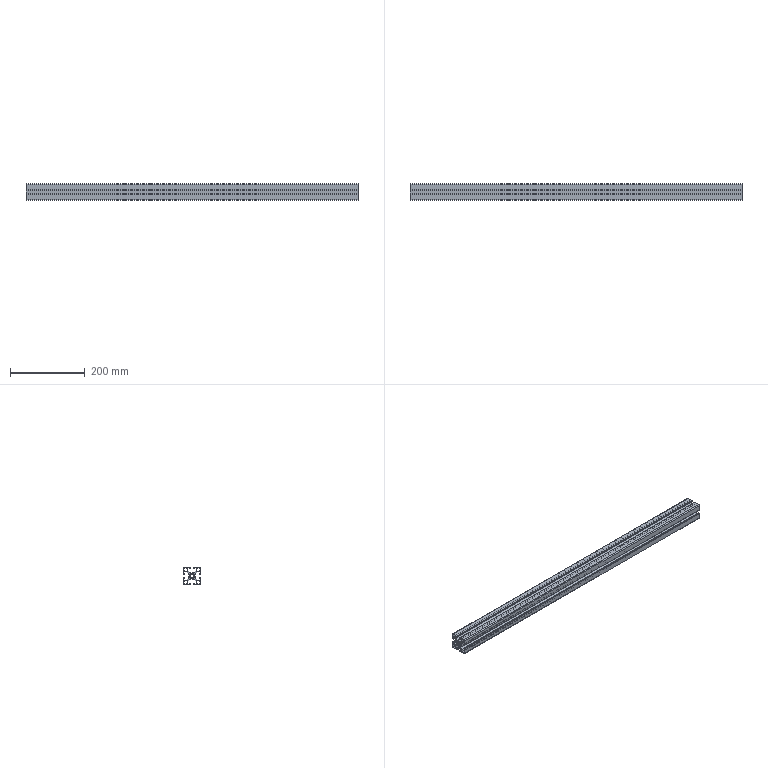Part | SolidWorks | features WeldMemberFeat 1, WeldmentFeature 1 | 1 solid | 135 faces | box 890 x 45 x 45 mm | volume 616138 mm3 | plane 118 | cylinder 17 | commonest cylinder face diameters 10 x9 3 x4 5 x4